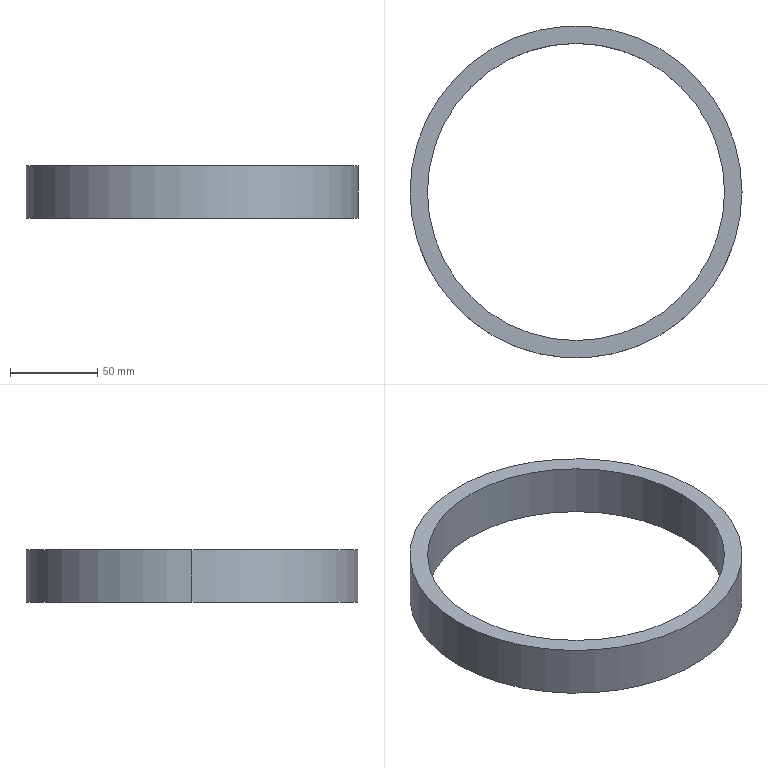Part | SolidWorks | features Extrusion 1 | 1 solid | 6 faces | box 190 x 190 x 30 mm | volume 169646 mm3 | cylinder 4 | plane 2 | commonest cylinder face diameters 170 x2 190 x2
STEP:
#1=CARTESIAN_POINT('',(-85.,0.,30.));
#2=VERTEX_POINT('',#1);
#3=CARTESIAN_POINT('',(85.,0.,30.));
#4=VERTEX_POINT('',#3);
#5=CARTESIAN_POINT('',(0.,0.,30.));
#6=DIRECTION('',(0.,0.,1.));
#7=DIRECTION('',(1.,0.,0.));
#8=AXIS2_PLACEMENT_3D('',#5,#6,#7);
#9=CIRCLE('',#8,85.);
#10=EDGE_CURVE('',#2,#4,#9,.T.);
#11=ORIENTED_EDGE('',*,*,#10,.T.);
#12=CARTESIAN_POINT('',(85.,0.,0.));
#13=VERTEX_POINT('',#12);
#14=CARTESIAN_POINT('',(85.,0.,30.));
#15=DIRECTION('',(0.,0.,-1.));
#16=VECTOR('',#15,1000.);
#17=LINE('',#14,#16);
#18=EDGE_CURVE('',#4,#13,#17,.T.);
#19=ORIENTED_EDGE('',*,*,#18,.T.);
#20=CARTESIAN_POINT('',(-85.,0.,0.));
#21=VERTEX_POINT('',#20);
#22=CARTESIAN_POINT('',(0.,0.,0.));
#23=DIRECTION('',(0.,0.,1.));
#24=DIRECTION('',(1.,0.,0.));
#25=AXIS2_PLACEMENT_3D('',#22,#23,#24);
#26=CIRCLE('',#25,85.);
#27=EDGE_CURVE('',#21,#13,#26,.T.);
#28=ORIENTED_EDGE('',*,*,#27,.F.);
#29=CARTESIAN_POINT('',(-85.,0.,30.));
#30=DIRECTION('',(0.,0.,-1.));
#31=VECTOR('',#30,1000.);
#32=LINE('',#29,#31);
#33=EDGE_CURVE('',#2,#21,#32,.T.);
#34=ORIENTED_EDGE('',*,*,#33,.F.);
#35=EDGE_LOOP('',(#11,#19,#28,#34));
#36=FACE_OUTER_BOUND('',#35,.T.);
#37=CARTESIAN_POINT('',(0.,0.,30.));
#38=DIRECTION('',(0.,0.,-1.));
#39=DIRECTION('',(-1.,0.,0.));
#40=AXIS2_PLACEMENT_3D('',#37,#38,#39);
#41=CYLINDRICAL_SURFACE('',#40,85.);
#42=ADVANCED_FACE('',(#36),#41,.F.);
#43=CARTESIAN_POINT('',(95.,0.,30.));
#44=VERTEX_POINT('',#43);
#45=CARTESIAN_POINT('',(-95.,0.,30.));
#46=VERTEX_POINT('',#45);
#47=CARTESIAN_POINT('',(0.,0.,30.));
#48=DIRECTION('',(0.,0.,1.));
#49=DIRECTION('',(1.,0.,0.));
#50=AXIS2_PLACEMENT_3D('',#47,#48,#49);
#51=CIRCLE('',#50,95.);
#52=EDGE_CURVE('',#44,#46,#51,.T.);
#53=ORIENTED_EDGE('',*,*,#52,.F.);
#54=CARTESIAN_POINT('',(95.,0.,0.));
#55=VERTEX_POINT('',#54);
#56=CARTESIAN_POINT('',(95.,0.,30.));
#57=DIRECTION('',(0.,0.,-1.));
#58=VECTOR('',#57,1000.);
#59=LINE('',#56,#58);
#60=EDGE_CURVE('',#44,#55,#59,.T.);
#61=ORIENTED_EDGE('',*,*,#60,.T.);
#62=CARTESIAN_POINT('',(-95.,0.,0.));
#63=VERTEX_POINT('',#62);
#64=CARTESIAN_POINT('',(0.,0.,0.));
#65=DIRECTION('',(0.,0.,1.));
#66=DIRECTION('',(1.,0.,0.));
#67=AXIS2_PLACEMENT_3D('',#64,#65,#66);
#68=CIRCLE('',#67,95.);
#69=EDGE_CURVE('',#55,#63,#68,.T.);
#70=ORIENTED_EDGE('',*,*,#69,.T.);
#71=CARTESIAN_POINT('',(-95.,0.,30.));
#72=DIRECTION('',(0.,0.,-1.));
#73=VECTOR('',#72,1000.);
#74=LINE('',#71,#73);
#75=EDGE_CURVE('',#46,#63,#74,.T.);
#76=ORIENTED_EDGE('',*,*,#75,.F.);
#77=EDGE_LOOP('',(#53,#61,#70,#76));
#78=FACE_OUTER_BOUND('',#77,.T.);
#79=CARTESIAN_POINT('',(0.,0.,30.));
#80=DIRECTION('',(0.,0.,-1.));
#81=DIRECTION('',(-1.,0.,0.));
#82=AXIS2_PLACEMENT_3D('',#79,#80,#81);
#83=CYLINDRICAL_SURFACE('',#82,95.);
#84=ADVANCED_FACE('',(#78),#83,.T.);
#85=CARTESIAN_POINT('',(0.,0.,30.));
#86=DIRECTION('',(0.,0.,1.));
#87=DIRECTION('',(1.,0.,0.));
#88=AXIS2_PLACEMENT_3D('',#85,#86,#87);
#89=CIRCLE('',#88,95.);
#90=EDGE_CURVE('',#46,#44,#89,.T.);
#91=ORIENTED_EDGE('',*,*,#90,.T.);
#92=ORIENTED_EDGE('',*,*,#52,.T.);
#93=EDGE_LOOP('',(#91,#92));
#94=FACE_OUTER_BOUND('',#93,.T.);
#95=ORIENTED_EDGE('',*,*,#10,.F.);
#96=CARTESIAN_POINT('',(0.,0.,30.));
#97=DIRECTION('',(0.,0.,1.));
#98=DIRECTION('',(1.,0.,0.));
#99=AXIS2_PLACEMENT_3D('',#96,#97,#98);
#100=CIRCLE('',#99,85.);
#101=EDGE_CURVE('',#4,#2,#100,.T.);
#102=ORIENTED_EDGE('',*,*,#101,.F.);
#103=EDGE_LOOP('',(#95,#102));
#104=FACE_BOUND('',#103,.T.);
#105=CARTESIAN_POINT('',(0.,0.,30.));
#106=DIRECTION('',(0.,0.,1.));
#107=DIRECTION('',(1.,0.,0.));
#108=AXIS2_PLACEMENT_3D('',#105,#106,#107);
#109=PLANE('',#108);
#110=ADVANCED_FACE('',(#94,#104),#109,.T.);
#111=CARTESIAN_POINT('',(0.,0.,0.));
#112=DIRECTION('',(0.,0.,1.));
#113=DIRECTION('',(1.,0.,0.));
#114=AXIS2_PLACEMENT_3D('',#111,#112,#113);
#115=CIRCLE('',#114,95.);
#116=EDGE_CURVE('',#63,#55,#115,.T.);
#117=ORIENTED_EDGE('',*,*,#116,.F.);
#118=ORIENTED_EDGE('',*,*,#69,.F.);
#119=EDGE_LOOP('',(#117,#118));
#120=FACE_OUTER_BOUND('',#119,.T.);
#121=ORIENTED_EDGE('',*,*,#27,.T.);
#122=CARTESIAN_POINT('',(0.,0.,0.));
#123=DIRECTION('',(0.,0.,1.));
#124=DIRECTION('',(1.,0.,0.));
#125=AXIS2_PLACEMENT_3D('',#122,#123,#124);
#126=CIRCLE('',#125,85.);
#127=EDGE_CURVE('',#13,#21,#126,.T.);
#128=ORIENTED_EDGE('',*,*,#127,.T.);
#129=EDGE_LOOP('',(#121,#128));
#130=FACE_BOUND('',#129,.T.);
#131=CARTESIAN_POINT('',(0.,0.,0.));
#132=DIRECTION('',(0.,0.,1.));
#133=DIRECTION('',(1.,0.,0.));
#134=AXIS2_PLACEMENT_3D('',#131,#132,#133);
#135=PLANE('',#134);
#136=ADVANCED_FACE('',(#120,#130),#135,.F.);
#137=ORIENTED_EDGE('',*,*,#60,.F.);
#138=ORIENTED_EDGE('',*,*,#90,.F.);
#139=ORIENTED_EDGE('',*,*,#75,.T.);
#140=ORIENTED_EDGE('',*,*,#116,.T.);
#141=EDGE_LOOP('',(#137,#138,#139,#140));
#142=FACE_OUTER_BOUND('',#141,.T.);
#143=CARTESIAN_POINT('',(0.,0.,30.));
#144=DIRECTION('',(0.,0.,-1.));
#145=DIRECTION('',(-1.,0.,0.));
#146=AXIS2_PLACEMENT_3D('',#143,#144,#145);
#147=CYLINDRICAL_SURFACE('',#146,95.);
#148=ADVANCED_FACE('',(#142),#147,.T.);
#149=ORIENTED_EDGE('',*,*,#18,.F.);
#150=ORIENTED_EDGE('',*,*,#101,.T.);
#151=ORIENTED_EDGE('',*,*,#33,.T.);
#152=ORIENTED_EDGE('',*,*,#127,.F.);
#153=EDGE_LOOP('',(#149,#150,#151,#152));
#154=FACE_OUTER_BOUND('',#153,.T.);
#155=CARTESIAN_POINT('',(0.,0.,30.));
#156=DIRECTION('',(0.,0.,-1.));
#157=DIRECTION('',(-1.,0.,0.));
#158=AXIS2_PLACEMENT_3D('',#155,#156,#157);
#159=CYLINDRICAL_SURFACE('',#158,85.);
#160=ADVANCED_FACE('',(#154),#159,.F.);
#161=CLOSED_SHELL('',(#42,#84,#110,#136,#148,#160));
#162=MANIFOLD_SOLID_BREP('',#161);
#163=CARTESIAN_POINT('',(0.,0.,0.));
#164=DIRECTION('',(0.,0.,1.));
#165=DIRECTION('',(1.,0.,0.));
#166=AXIS2_PLACEMENT_3D('',#163,#164,#165);
#167=(LENGTH_UNIT()NAMED_UNIT(*)SI_UNIT(.MILLI.,.METRE.));
#168=UNCERTAINTY_MEASURE_WITH_UNIT(LENGTH_MEASURE(0.00001),#167,'','');
#169=(NAMED_UNIT(*)PLANE_ANGLE_UNIT()SI_UNIT($,.RADIAN.));
#170=(NAMED_UNIT(*)SI_UNIT($,.STERADIAN.)SOLID_ANGLE_UNIT());
#171=(GEOMETRIC_REPRESENTATION_CONTEXT(3)GLOBAL_UNCERTAINTY_ASSIGNED_CONTEXT((#168))GLOBAL_UNIT_ASSIGNED_CONTEXT((#167,#169,#170))REPRESENTATION_CONTEXT('',''));
#172=ADVANCED_BREP_SHAPE_REPRESENTATION('',(#162,#166),#171);